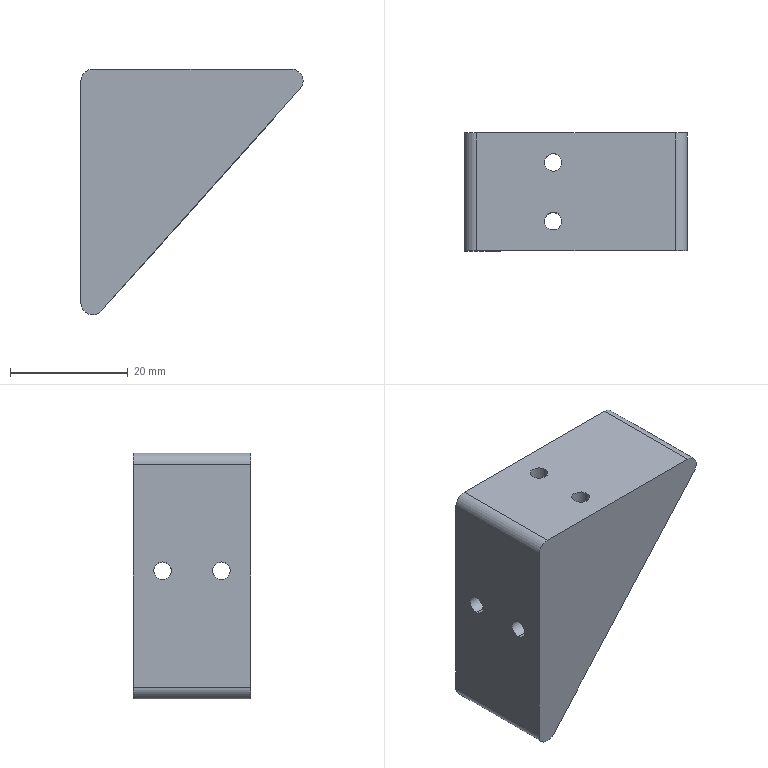Part | SolidWorks | features ICE 2, Extrusion 1, Fillet 1 | 1 solid | 25 faces | box 37.777 x 20 x 41.764 mm | volume 17216 mm3 | cylinder 20 | plane 5 | commonest cylinder face diameters 3 x16 4 x4
STEP:
#1=CARTESIAN_POINT('',(13.5,5.,-29.907));
#2=VERTEX_POINT('',#1);
#3=CARTESIAN_POINT('',(16.5,5.,-26.552));
#4=VERTEX_POINT('',#3);
#5=CARTESIAN_POINT('',(13.5,5.,-29.907));
#6=CARTESIAN_POINT('',(13.5,2.,-29.907));
#7=CARTESIAN_POINT('',(16.5,2.,-26.552));
#8=CARTESIAN_POINT('',(16.5,5.,-26.552));
#9=(BOUNDED_CURVE()B_SPLINE_CURVE(3,(#5,#6,#7,#8),.UNSPECIFIED.,.F.,.F.)B_SPLINE_CURVE_WITH_KNOTS((4,4),(3.142,6.283),.UNSPECIFIED.)CURVE()GEOMETRIC_REPRESENTATION_ITEM()RATIONAL_B_SPLINE_CURVE((1.,0.3333,0.3333,1.))REPRESENTATION_ITEM(''));
#10=EDGE_CURVE('',#2,#4,#9,.T.);
#11=ORIENTED_EDGE('',*,*,#10,.F.);
#12=CARTESIAN_POINT('',(13.5,5.,-21.5));
#13=VERTEX_POINT('',#12);
#14=CARTESIAN_POINT('',(13.5,5.,-41.764));
#15=DIRECTION('',(0.,0.,1.));
#16=VECTOR('',#15,1000.);
#17=LINE('',#14,#16);
#18=EDGE_CURVE('',#2,#13,#17,.T.);
#19=ORIENTED_EDGE('',*,*,#18,.T.);
#20=CARTESIAN_POINT('',(15.,3.5,-20.));
#21=VERTEX_POINT('',#20);
#22=CARTESIAN_POINT('',(15.,3.5,-20.));
#23=CARTESIAN_POINT('',(14.121,3.5,-20.879));
#24=CARTESIAN_POINT('',(13.5,4.121,-21.5));
#25=CARTESIAN_POINT('',(13.5,5.,-21.5));
#26=(BOUNDED_CURVE()B_SPLINE_CURVE(3,(#22,#23,#24,#25),.UNSPECIFIED.,.F.,.F.)B_SPLINE_CURVE_WITH_KNOTS((4,4),(4.712,6.283),.UNSPECIFIED.)CURVE()GEOMETRIC_REPRESENTATION_ITEM()RATIONAL_B_SPLINE_CURVE((1.,0.8047,0.8047,1.))REPRESENTATION_ITEM(''));
#27=EDGE_CURVE('',#21,#13,#26,.T.);
#28=ORIENTED_EDGE('',*,*,#27,.F.);
#29=CARTESIAN_POINT('',(16.5,5.,-21.5));
#30=VERTEX_POINT('',#29);
#31=CARTESIAN_POINT('',(16.5,5.,-21.5));
#32=CARTESIAN_POINT('',(16.5,4.121,-21.5));
#33=CARTESIAN_POINT('',(15.879,3.5,-20.879));
#34=CARTESIAN_POINT('',(15.,3.5,-20.));
#35=(BOUNDED_CURVE()B_SPLINE_CURVE(3,(#31,#32,#33,#34),.UNSPECIFIED.,.F.,.F.)B_SPLINE_CURVE_WITH_KNOTS((4,4),(3.142,4.712),.UNSPECIFIED.)CURVE()GEOMETRIC_REPRESENTATION_ITEM()RATIONAL_B_SPLINE_CURVE((1.,0.8047,0.8047,1.))REPRESENTATION_ITEM(''));
#36=EDGE_CURVE('',#30,#21,#35,.T.);
#37=ORIENTED_EDGE('',*,*,#36,.F.);
#38=CARTESIAN_POINT('',(16.5,5.,-41.764));
#39=DIRECTION('',(0.,0.,1.));
#40=VECTOR('',#39,1000.);
#41=LINE('',#38,#40);
#42=EDGE_CURVE('',#4,#30,#41,.T.);
#43=ORIENTED_EDGE('',*,*,#42,.F.);
#44=EDGE_LOOP('',(#11,#19,#28,#37,#43));
#45=FACE_OUTER_BOUND('',#44,.T.);
#46=CARTESIAN_POINT('',(15.,5.,-41.764));
#47=DIRECTION('',(0.,0.,1.));
#48=DIRECTION('',(1.,0.,0.));
#49=AXIS2_PLACEMENT_3D('',#46,#47,#48);
#50=CYLINDRICAL_SURFACE('',#49,1.5);
#51=ADVANCED_FACE('',(#45),#50,.F.);
#52=CARTESIAN_POINT('',(13.5,5.,-18.5));
#53=VERTEX_POINT('',#52);
#54=CARTESIAN_POINT('',(13.5,5.,-18.5));
#55=CARTESIAN_POINT('',(13.5,4.121,-18.5));
#56=CARTESIAN_POINT('',(14.121,3.5,-19.121));
#57=CARTESIAN_POINT('',(15.,3.5,-20.));
#58=(BOUNDED_CURVE()B_SPLINE_CURVE(3,(#54,#55,#56,#57),.UNSPECIFIED.,.F.,.F.)B_SPLINE_CURVE_WITH_KNOTS((4,4),(0.,1.571),.UNSPECIFIED.)CURVE()GEOMETRIC_REPRESENTATION_ITEM()RATIONAL_B_SPLINE_CURVE((1.,0.8047,0.8047,1.))REPRESENTATION_ITEM(''));
#59=EDGE_CURVE('',#53,#21,#58,.T.);
#60=ORIENTED_EDGE('',*,*,#59,.F.);
#61=CARTESIAN_POINT('',(13.5,5.,0.));
#62=VERTEX_POINT('',#61);
#63=CARTESIAN_POINT('',(13.5,5.,-41.764));
#64=DIRECTION('',(0.,0.,1.));
#65=VECTOR('',#64,1000.);
#66=LINE('',#63,#65);
#67=EDGE_CURVE('',#53,#62,#66,.T.);
#68=ORIENTED_EDGE('',*,*,#67,.T.);
#69=CARTESIAN_POINT('',(16.5,5.,0.));
#70=VERTEX_POINT('',#69);
#71=CARTESIAN_POINT('',(15.,5.,0.));
#72=DIRECTION('',(0.,0.,1.));
#73=DIRECTION('',(1.,0.,0.));
#74=AXIS2_PLACEMENT_3D('',#71,#72,#73);
#75=CIRCLE('',#74,1.5);
#76=EDGE_CURVE('',#62,#70,#75,.T.);
#77=ORIENTED_EDGE('',*,*,#76,.T.);
#78=CARTESIAN_POINT('',(16.5,5.,-18.5));
#79=VERTEX_POINT('',#78);
#80=CARTESIAN_POINT('',(16.5,5.,-41.764));
#81=DIRECTION('',(0.,0.,1.));
#82=VECTOR('',#81,1000.);
#83=LINE('',#80,#82);
#84=EDGE_CURVE('',#79,#70,#83,.T.);
#85=ORIENTED_EDGE('',*,*,#84,.F.);
#86=CARTESIAN_POINT('',(15.,3.5,-20.));
#87=CARTESIAN_POINT('',(15.879,3.5,-19.121));
#88=CARTESIAN_POINT('',(16.5,4.121,-18.5));
#89=CARTESIAN_POINT('',(16.5,5.,-18.5));
#90=(BOUNDED_CURVE()B_SPLINE_CURVE(3,(#86,#87,#88,#89),.UNSPECIFIED.,.F.,.F.)B_SPLINE_CURVE_WITH_KNOTS((4,4),(1.571,3.142),.UNSPECIFIED.)CURVE()GEOMETRIC_REPRESENTATION_ITEM()RATIONAL_B_SPLINE_CURVE((1.,0.8047,0.8047,1.))REPRESENTATION_ITEM(''));
#91=EDGE_CURVE('',#21,#79,#90,.T.);
#92=ORIENTED_EDGE('',*,*,#91,.F.);
#93=EDGE_LOOP('',(#60,#68,#77,#85,#92));
#94=FACE_OUTER_BOUND('',#93,.T.);
#95=CARTESIAN_POINT('',(15.,5.,-41.764));
#96=DIRECTION('',(0.,0.,1.));
#97=DIRECTION('',(1.,0.,0.));
#98=AXIS2_PLACEMENT_3D('',#95,#96,#97);
#99=CYLINDRICAL_SURFACE('',#98,1.5);
#100=ADVANCED_FACE('',(#94),#99,.F.);
#101=CARTESIAN_POINT('',(13.5,15.,-29.907));
#102=VERTEX_POINT('',#101);
#103=CARTESIAN_POINT('',(16.5,15.,-26.552));
#104=VERTEX_POINT('',#103);
#105=CARTESIAN_POINT('',(13.5,15.,-29.907));
#106=CARTESIAN_POINT('',(13.5,12.,-29.907));
#107=CARTESIAN_POINT('',(16.5,12.,-26.552));
#108=CARTESIAN_POINT('',(16.5,15.,-26.552));
#109=(BOUNDED_CURVE()B_SPLINE_CURVE(3,(#105,#106,#107,#108),.UNSPECIFIED.,.F.,.F.)B_SPLINE_CURVE_WITH_KNOTS((4,4),(3.142,6.283),.UNSPECIFIED.)CURVE()GEOMETRIC_REPRESENTATION_ITEM()RATIONAL_B_SPLINE_CURVE((1.,0.3333,0.3333,1.))REPRESENTATION_ITEM(''));
#110=EDGE_CURVE('',#102,#104,#109,.T.);
#111=ORIENTED_EDGE('',*,*,#110,.F.);
#112=CARTESIAN_POINT('',(13.5,15.,-21.5));
#113=VERTEX_POINT('',#112);
#114=CARTESIAN_POINT('',(13.5,15.,-41.764));
#115=DIRECTION('',(0.,0.,1.));
#116=VECTOR('',#115,1000.);
#117=LINE('',#114,#116);
#118=EDGE_CURVE('',#102,#113,#117,.T.);
#119=ORIENTED_EDGE('',*,*,#118,.T.);
#120=CARTESIAN_POINT('',(15.,13.5,-20.));
#121=VERTEX_POINT('',#120);
#122=CARTESIAN_POINT('',(15.,13.5,-20.));
#123=CARTESIAN_POINT('',(14.121,13.5,-20.879));
#124=CARTESIAN_POINT('',(13.5,14.121,-21.5));
#125=CARTESIAN_POINT('',(13.5,15.,-21.5));
#126=(BOUNDED_CURVE()B_SPLINE_CURVE(3,(#122,#123,#124,#125),.UNSPECIFIED.,.F.,.F.)B_SPLINE_CURVE_WITH_KNOTS((4,4),(4.712,6.283),.UNSPECIFIED.)CURVE()GEOMETRIC_REPRESENTATION_ITEM()RATIONAL_B_SPLINE_CURVE((1.,0.8047,0.8047,1.))REPRESENTATION_ITEM(''));
#127=EDGE_CURVE('',#121,#113,#126,.T.);
#128=ORIENTED_EDGE('',*,*,#127,.F.);
#129=CARTESIAN_POINT('',(16.5,15.,-21.5));
#130=VERTEX_POINT('',#129);
#131=CARTESIAN_POINT('',(16.5,15.,-21.5));
#132=CARTESIAN_POINT('',(16.5,14.121,-21.5));
#133=CARTESIAN_POINT('',(15.879,13.5,-20.879));
#134=CARTESIAN_POINT('',(15.,13.5,-20.));
#135=(BOUNDED_CURVE()B_SPLINE_CURVE(3,(#131,#132,#133,#134),.UNSPECIFIED.,.F.,.F.)B_SPLINE_CURVE_WITH_KNOTS((4,4),(3.142,4.712),.UNSPECIFIED.)CURVE()GEOMETRIC_REPRESENTATION_ITEM()RATIONAL_B_SPLINE_CURVE((1.,0.8047,0.8047,1.))REPRESENTATION_ITEM(''));
#136=EDGE_CURVE('',#130,#121,#135,.T.);
#137=ORIENTED_EDGE('',*,*,#136,.F.);
#138=CARTESIAN_POINT('',(16.5,15.,-41.764));
#139=DIRECTION('',(0.,0.,1.));
#140=VECTOR('',#139,1000.);
#141=LINE('',#138,#140);
#142=EDGE_CURVE('',#104,#130,#141,.T.);
#143=ORIENTED_EDGE('',*,*,#142,.F.);
#144=EDGE_LOOP('',(#111,#119,#128,#137,#143));
#145=FACE_OUTER_BOUND('',#144,.T.);
#146=CARTESIAN_POINT('',(15.,15.,-41.764));
#147=DIRECTION('',(0.,0.,1.));
#148=DIRECTION('',(1.,0.,0.));
#149=AXIS2_PLACEMENT_3D('',#146,#147,#148);
#150=CYLINDRICAL_SURFACE('',#149,1.5);
#151=ADVANCED_FACE('',(#145),#150,.F.);
#152=CARTESIAN_POINT('',(13.5,15.,-18.5));
#153=VERTEX_POINT('',#152);
#154=CARTESIAN_POINT('',(13.5,15.,-18.5));
#155=CARTESIAN_POINT('',(13.5,14.121,-18.5));
#156=CARTESIAN_POINT('',(14.121,13.5,-19.121));
#157=CARTESIAN_POINT('',(15.,13.5,-20.));
#158=(BOUNDED_CURVE()B_SPLINE_CURVE(3,(#154,#155,#156,#157),.UNSPECIFIED.,.F.,.F.)B_SPLINE_CURVE_WITH_KNOTS((4,4),(0.,1.571),.UNSPECIFIED.)CURVE()GEOMETRIC_REPRESENTATION_ITEM()RATIONAL_B_SPLINE_CURVE((1.,0.8047,0.8047,1.))REPRESENTATION_ITEM(''));
#159=EDGE_CURVE('',#153,#121,#158,.T.);
#160=ORIENTED_EDGE('',*,*,#159,.F.);
#161=CARTESIAN_POINT('',(13.5,15.,0.));
#162=VERTEX_POINT('',#161);
#163=CARTESIAN_POINT('',(13.5,15.,-41.764));
#164=DIRECTION('',(0.,0.,1.));
#165=VECTOR('',#164,1000.);
#166=LINE('',#163,#165);
#167=EDGE_CURVE('',#153,#162,#166,.T.);
#168=ORIENTED_EDGE('',*,*,#167,.T.);
#169=CARTESIAN_POINT('',(16.5,15.,0.));
#170=VERTEX_POINT('',#169);
#171=CARTESIAN_POINT('',(15.,15.,0.));
#172=DIRECTION('',(0.,0.,1.));
#173=DIRECTION('',(1.,0.,0.));
#174=AXIS2_PLACEMENT_3D('',#171,#172,#173);
#175=CIRCLE('',#174,1.5);
#176=EDGE_CURVE('',#162,#170,#175,.T.);
#177=ORIENTED_EDGE('',*,*,#176,.T.);
#178=CARTESIAN_POINT('',(16.5,15.,-18.5));
#179=VERTEX_POINT('',#178);
#180=CARTESIAN_POINT('',(16.5,15.,-41.764));
#181=DIRECTION('',(0.,0.,1.));
#182=VECTOR('',#181,1000.);
#183=LINE('',#180,#182);
#184=EDGE_CURVE('',#179,#170,#183,.T.);
#185=ORIENTED_EDGE('',*,*,#184,.F.);
#186=CARTESIAN_POINT('',(15.,13.5,-20.));
#187=CARTESIAN_POINT('',(15.879,13.5,-19.121));
#188=CARTESIAN_POINT('',(16.5,14.121,-18.5));
#189=CARTESIAN_POINT('',(16.5,15.,-18.5));
#190=(BOUNDED_CURVE()B_SPLINE_CURVE(3,(#186,#187,#188,#189),.UNSPECIFIED.,.F.,.F.)B_SPLINE_CURVE_WITH_KNOTS((4,4),(1.571,3.142),.UNSPECIFIED.)CURVE()GEOMETRIC_REPRESENTATION_ITEM()RATIONAL_B_SPLINE_CURVE((1.,0.8047,0.8047,1.))REPRESENTATION_ITEM(''));
#191=EDGE_CURVE('',#121,#179,#190,.T.);
#192=ORIENTED_EDGE('',*,*,#191,.F.);
#193=EDGE_LOOP('',(#160,#168,#177,#185,#192));
#194=FACE_OUTER_BOUND('',#193,.T.);
#195=CARTESIAN_POINT('',(15.,15.,-41.764));
#196=DIRECTION('',(0.,0.,1.));
#197=DIRECTION('',(1.,0.,0.));
#198=AXIS2_PLACEMENT_3D('',#195,#196,#197);
#199=CYLINDRICAL_SURFACE('',#198,1.5);
#200=ADVANCED_FACE('',(#194),#199,.F.);
#201=CARTESIAN_POINT('',(21.019,15.,-21.5));
#202=VERTEX_POINT('',#201);
#203=CARTESIAN_POINT('',(23.702,15.,-18.5));
#204=VERTEX_POINT('',#203);
#205=CARTESIAN_POINT('',(21.019,15.,-21.5));
#206=CARTESIAN_POINT('',(21.019,12.,-21.5));
#207=CARTESIAN_POINT('',(23.702,12.,-18.5));
#208=CARTESIAN_POINT('',(23.702,15.,-18.5));
#209=(BOUNDED_CURVE()B_SPLINE_CURVE(3,(#205,#206,#207,#208),.UNSPECIFIED.,.F.,.T.)B_SPLINE_CURVE_WITH_KNOTS((4,4),(0.,3.142),.UNSPECIFIED.)CURVE()GEOMETRIC_REPRESENTATION_ITEM()RATIONAL_B_SPLINE_CURVE((1.,0.3333,0.3333,1.))REPRESENTATION_ITEM(''));
#210=EDGE_CURVE('',#202,#204,#209,.T.);
#211=ORIENTED_EDGE('',*,*,#210,.F.);
#212=CARTESIAN_POINT('',(37.777,15.,-21.5));
#213=DIRECTION('',(-1.,0.,0.));
#214=VECTOR('',#213,1000.);
#215=LINE('',#212,#214);
#216=EDGE_CURVE('',#202,#130,#215,.T.);
#217=ORIENTED_EDGE('',*,*,#216,.T.);
#218=ORIENTED_EDGE('',*,*,#136,.T.);
#219=ORIENTED_EDGE('',*,*,#191,.T.);
#220=CARTESIAN_POINT('',(37.777,15.,-18.5));
#221=DIRECTION('',(-1.,0.,0.));
#222=VECTOR('',#221,1000.);
#223=LINE('',#220,#222);
#224=EDGE_CURVE('',#204,#179,#223,.T.);
#225=ORIENTED_EDGE('',*,*,#224,.F.);
#226=EDGE_LOOP('',(#211,#217,#218,#219,#225));
#227=FACE_OUTER_BOUND('',#226,.T.);
#228=CARTESIAN_POINT('',(37.777,15.,-20.));
#229=DIRECTION('',(-1.,0.,0.));
#230=DIRECTION('',(0.,0.,1.));
#231=AXIS2_PLACEMENT_3D('',#228,#229,#230);
#232=CYLINDRICAL_SURFACE('',#231,1.5);
#233=ADVANCED_FACE('',(#227),#232,.F.);
#234=CARTESIAN_POINT('',(21.019,5.,-21.5));
#235=VERTEX_POINT('',#234);
#236=CARTESIAN_POINT('',(23.702,5.,-18.5));
#237=VERTEX_POINT('',#236);
#238=CARTESIAN_POINT('',(21.019,5.,-21.5));
#239=CARTESIAN_POINT('',(21.019,2.,-21.5));
#240=CARTESIAN_POINT('',(23.702,2.,-18.5));
#241=CARTESIAN_POINT('',(23.702,5.,-18.5));
#242=(BOUNDED_CURVE()B_SPLINE_CURVE(3,(#238,#239,#240,#241),.UNSPECIFIED.,.F.,.F.)B_SPLINE_CURVE_WITH_KNOTS((4,4),(0.,3.142),.UNSPECIFIED.)CURVE()GEOMETRIC_REPRESENTATION_ITEM()RATIONAL_B_SPLINE_CURVE((1.,0.3333,0.3333,1.))REPRESENTATION_ITEM(''));
#243=EDGE_CURVE('',#235,#237,#242,.T.);
#244=ORIENTED_EDGE('',*,*,#243,.F.);
#245=CARTESIAN_POINT('',(37.777,5.,-21.5));
#246=DIRECTION('',(-1.,0.,0.));
#247=VECTOR('',#246,1000.);
#248=LINE('',#245,#247);
#249=EDGE_CURVE('',#235,#30,#248,.T.);
#250=ORIENTED_EDGE('',*,*,#249,.T.);
#251=ORIENTED_EDGE('',*,*,#36,.T.);
#252=ORIENTED_EDGE('',*,*,#91,.T.);
#253=CARTESIAN_POINT('',(37.777,5.,-18.5));
#254=DIRECTION('',(-1.,0.,0.));
#255=VECTOR('',#254,1000.);
#256=LINE('',#253,#255);
#257=EDGE_CURVE('',#237,#79,#256,.T.);
#258=ORIENTED_EDGE('',*,*,#257,.F.);
#259=EDGE_LOOP('',(#244,#250,#251,#252,#258));
#260=FACE_OUTER_BOUND('',#259,.T.);
#261=CARTESIAN_POINT('',(37.777,5.,-20.));
#262=DIRECTION('',(-1.,0.,0.));
#263=DIRECTION('',(0.,0.,1.));
#264=AXIS2_PLACEMENT_3D('',#261,#262,#263);
#265=CYLINDRICAL_SURFACE('',#264,1.5);
#266=ADVANCED_FACE('',(#260),#265,.F.);
#267=CARTESIAN_POINT('',(2.,20.,-41.764));
#268=VERTEX_POINT('',#267);
#269=CARTESIAN_POINT('',(0.,20.,-39.764));
#270=VERTEX_POINT('',#269);
#271=CARTESIAN_POINT('',(2.,20.,-39.764));
#272=DIRECTION('',(0.,1.,0.));
#273=DIRECTION('',(0.,0.,-1.));
#274=AXIS2_PLACEMENT_3D('',#271,#272,#273);
#275=CIRCLE('',#274,2.);
#276=EDGE_CURVE('',#268,#270,#275,.T.);
#277=ORIENTED_EDGE('',*,*,#276,.F.);
#278=CARTESIAN_POINT('',(2.,0.,-41.764));
#279=VERTEX_POINT('',#278);
#280=CARTESIAN_POINT('',(2.,20.,-41.764));
#281=DIRECTION('',(0.,-1.,0.));
#282=VECTOR('',#281,1000.);
#283=LINE('',#280,#282);
#284=EDGE_CURVE('',#268,#279,#283,.T.);
#285=ORIENTED_EDGE('',*,*,#284,.T.);
#286=CARTESIAN_POINT('',(0.,0.,-39.764));
#287=VERTEX_POINT('',#286);
#288=CARTESIAN_POINT('',(2.,0.,-39.764));
#289=DIRECTION('',(0.,-1.,0.));
#290=DIRECTION('',(0.,0.,-1.));
#291=AXIS2_PLACEMENT_3D('',#288,#289,#290);
#292=CIRCLE('',#291,2.);
#293=EDGE_CURVE('',#287,#279,#292,.T.);
#294=ORIENTED_EDGE('',*,*,#293,.F.);
#295=CARTESIAN_POINT('',(0.,20.,-39.764));
#296=DIRECTION('',(0.,-1.,0.));
#297=VECTOR('',#296,1000.);
#298=LINE('',#295,#297);
#299=EDGE_CURVE('',#270,#287,#298,.T.);
#300=ORIENTED_EDGE('',*,*,#299,.F.);
#301=EDGE_LOOP('',(#277,#285,#294,#300));
#302=FACE_OUTER_BOUND('',#301,.T.);
#303=CARTESIAN_POINT('',(2.,20.,-39.764));
#304=DIRECTION('',(0.,-1.,0.));
#305=DIRECTION('',(0.,0.,-1.));
#306=AXIS2_PLACEMENT_3D('',#303,#304,#305);
#307=CYLINDRICAL_SURFACE('',#306,2.);
#308=ADVANCED_FACE('',(#302),#307,.T.);
#309=ORIENTED_EDGE('',*,*,#127,.T.);
#310=CARTESIAN_POINT('',(0.,15.,-21.5));
#311=VERTEX_POINT('',#310);
#312=CARTESIAN_POINT('',(37.777,15.,-21.5));
#313=DIRECTION('',(-1.,0.,0.));
#314=VECTOR('',#313,1000.);
#315=LINE('',#312,#314);
#316=EDGE_CURVE('',#113,#311,#315,.T.);
#317=ORIENTED_EDGE('',*,*,#316,.T.);
#318=CARTESIAN_POINT('',(0.,15.,-18.5));
#319=VERTEX_POINT('',#318);
#320=CARTESIAN_POINT('',(0.,15.,-20.));
#321=DIRECTION('',(-1.,0.,0.));
#322=DIRECTION('',(0.,0.,1.));
#323=AXIS2_PLACEMENT_3D('',#320,#321,#322);
#324=CIRCLE('',#323,1.5);
#325=EDGE_CURVE('',#311,#319,#324,.T.);
#326=ORIENTED_EDGE('',*,*,#325,.T.);
#327=CARTESIAN_POINT('',(37.777,15.,-18.5));
#328=DIRECTION('',(-1.,0.,0.));
#329=VECTOR('',#328,1000.);
#330=LINE('',#327,#329);
#331=EDGE_CURVE('',#153,#319,#330,.T.);
#332=ORIENTED_EDGE('',*,*,#331,.F.);
#333=ORIENTED_EDGE('',*,*,#159,.T.);
#334=EDGE_LOOP('',(#309,#317,#326,#332,#333));
#335=FACE_OUTER_BOUND('',#334,.T.);
#336=CARTESIAN_POINT('',(37.777,15.,-20.));
#337=DIRECTION('',(-1.,0.,0.));
#338=DIRECTION('',(0.,0.,1.));
#339=AXIS2_PLACEMENT_3D('',#336,#337,#338);
#340=CYLINDRICAL_SURFACE('',#339,1.5);
#341=ADVANCED_FACE('',(#335),#340,.F.);
#342=ORIENTED_EDGE('',*,*,#27,.T.);
#343=CARTESIAN_POINT('',(0.,5.,-21.5));
#344=VERTEX_POINT('',#343);
#345=CARTESIAN_POINT('',(37.777,5.,-21.5));
#346=DIRECTION('',(-1.,0.,0.));
#347=VECTOR('',#346,1000.);
#348=LINE('',#345,#347);
#349=EDGE_CURVE('',#13,#344,#348,.T.);
#350=ORIENTED_EDGE('',*,*,#349,.T.);
#351=CARTESIAN_POINT('',(0.,5.,-18.5));
#352=VERTEX_POINT('',#351);
#353=CARTESIAN_POINT('',(0.,5.,-20.));
#354=DIRECTION('',(-1.,0.,0.));
#355=DIRECTION('',(0.,0.,1.));
#356=AXIS2_PLACEMENT_3D('',#353,#354,#355);
#357=CIRCLE('',#356,1.5);
#358=EDGE_CURVE('',#344,#352,#357,.T.);
#359=ORIENTED_EDGE('',*,*,#358,.T.);
#360=CARTESIAN_POINT('',(37.777,5.,-18.5));
#361=DIRECTION('',(-1.,0.,0.));
#362=VECTOR('',#361,1000.);
#363=LINE('',#360,#362);
#364=EDGE_CURVE('',#53,#352,#363,.T.);
#365=ORIENTED_EDGE('',*,*,#364,.F.);
#366=ORIENTED_EDGE('',*,*,#59,.T.);
#367=EDGE_LOOP('',(#342,#350,#359,#365,#366));
#368=FACE_OUTER_BOUND('',#367,.T.);
#369=CARTESIAN_POINT('',(37.777,5.,-20.));
#370=DIRECTION('',(-1.,0.,0.));
#371=DIRECTION('',(0.,0.,1.));
#372=AXIS2_PLACEMENT_3D('',#369,#370,#371);
#373=CYLINDRICAL_SURFACE('',#372,1.5);
#374=ADVANCED_FACE('',(#368),#373,.F.);
#375=ORIENTED_EDGE('',*,*,#349,.F.);
#376=CARTESIAN_POINT('',(15.,6.5,-20.));
#377=VERTEX_POINT('',#376);
#378=CARTESIAN_POINT('',(13.5,5.,-21.5));
#379=CARTESIAN_POINT('',(13.5,5.879,-21.5));
#380=CARTESIAN_POINT('',(14.121,6.5,-20.879));
#381=CARTESIAN_POINT('',(15.,6.5,-20.));
#382=(BOUNDED_CURVE()B_SPLINE_CURVE(3,(#378,#379,#380,#381),.UNSPECIFIED.,.F.,.F.)B_SPLINE_CURVE_WITH_KNOTS((4,4),(0.,1.571),.UNSPECIFIED.)CURVE()GEOMETRIC_REPRESENTATION_ITEM()RATIONAL_B_SPLINE_CURVE((1.,0.8047,0.8047,1.))REPRESENTATION_ITEM(''));
#383=EDGE_CURVE('',#13,#377,#382,.T.);
#384=ORIENTED_EDGE('',*,*,#383,.T.);
#385=CARTESIAN_POINT('',(15.,6.5,-20.));
#386=CARTESIAN_POINT('',(14.121,6.5,-19.121));
#387=CARTESIAN_POINT('',(13.5,5.879,-18.5));
#388=CARTESIAN_POINT('',(13.5,5.,-18.5));
#389=(BOUNDED_CURVE()B_SPLINE_CURVE(3,(#385,#386,#387,#388),.UNSPECIFIED.,.F.,.F.)B_SPLINE_CURVE_WITH_KNOTS((4,4),(4.712,6.283),.UNSPECIFIED.)CURVE()GEOMETRIC_REPRESENTATION_ITEM()RATIONAL_B_SPLINE_CURVE((1.,0.8047,0.8047,1.))REPRESENTATION_ITEM(''));
#390=EDGE_CURVE('',#377,#53,#389,.T.);
#391=ORIENTED_EDGE('',*,*,#390,.T.);
#392=ORIENTED_EDGE('',*,*,#364,.T.);
#393=CARTESIAN_POINT('',(0.,5.,-20.));
#394=DIRECTION('',(-1.,0.,0.));
#395=DIRECTION('',(0.,0.,1.));
#396=AXIS2_PLACEMENT_3D('',#393,#394,#395);
#397=CIRCLE('',#396,1.5);
#398=EDGE_CURVE('',#352,#344,#397,.T.);
#399=ORIENTED_EDGE('',*,*,#398,.T.);
#400=EDGE_LOOP('',(#375,#384,#391,#392,#399));
#401=FACE_OUTER_BOUND('',#400,.T.);
#402=CARTESIAN_POINT('',(37.777,5.,-20.));
#403=DIRECTION('',(-1.,0.,0.));
#404=DIRECTION('',(0.,0.,1.));
#405=AXIS2_PLACEMENT_3D('',#402,#403,#404);
#406=CYLINDRICAL_SURFACE('',#405,1.5);
#407=ADVANCED_FACE('',(#401),#406,.F.);
#408=ORIENTED_EDGE('',*,*,#316,.F.);
#409=CARTESIAN_POINT('',(15.,16.5,-20.));
#410=VERTEX_POINT('',#409);
#411=CARTESIAN_POINT('',(13.5,15.,-21.5));
#412=CARTESIAN_POINT('',(13.5,15.879,-21.5));
#413=CARTESIAN_POINT('',(14.121,16.5,-20.879));
#414=CARTESIAN_POINT('',(15.,16.5,-20.));
#415=(BOUNDED_CURVE()B_SPLINE_CURVE(3,(#411,#412,#413,#414),.UNSPECIFIED.,.F.,.F.)B_SPLINE_CURVE_WITH_KNOTS((4,4),(0.,1.571),.UNSPECIFIED.)CURVE()GEOMETRIC_REPRESENTATION_ITEM()RATIONAL_B_SPLINE_CURVE((1.,0.8047,0.8047,1.))REPRESENTATION_ITEM(''));
#416=EDGE_CURVE('',#113,#410,#415,.T.);
#417=ORIENTED_EDGE('',*,*,#416,.T.);
#418=CARTESIAN_POINT('',(15.,16.5,-20.));
#419=CARTESIAN_POINT('',(14.121,16.5,-19.121));
#420=CARTESIAN_POINT('',(13.5,15.879,-18.5));
#421=CARTESIAN_POINT('',(13.5,15.,-18.5));
#422=(BOUNDED_CURVE()B_SPLINE_CURVE(3,(#418,#419,#420,#421),.UNSPECIFIED.,.F.,.F.)B_SPLINE_CURVE_WITH_KNOTS((4,4),(4.712,6.283),.UNSPECIFIED.)CURVE()GEOMETRIC_REPRESENTATION_ITEM()RATIONAL_B_SPLINE_CURVE((1.,0.8047,0.8047,1.))REPRESENTATION_ITEM(''));
#423=EDGE_CURVE('',#410,#153,#422,.T.);
#424=ORIENTED_EDGE('',*,*,#423,.T.);
#425=ORIENTED_EDGE('',*,*,#331,.T.);
#426=CARTESIAN_POINT('',(0.,15.,-20.));
#427=DIRECTION('',(-1.,0.,0.));
#428=DIRECTION('',(0.,0.,1.));
#429=AXIS2_PLACEMENT_3D('',#426,#427,#428);
#430=CIRCLE('',#429,1.5);
#431=EDGE_CURVE('',#319,#311,#430,.T.);
#432=ORIENTED_EDGE('',*,*,#431,.T.);
#433=EDGE_LOOP('',(#408,#417,#424,#425,#432));
#434=FACE_OUTER_BOUND('',#433,.T.);
#435=CARTESIAN_POINT('',(37.777,15.,-20.));
#436=DIRECTION('',(-1.,0.,0.));
#437=DIRECTION('',(0.,0.,1.));
#438=AXIS2_PLACEMENT_3D('',#435,#436,#437);
#439=CYLINDRICAL_SURFACE('',#438,1.5);
#440=ADVANCED_FACE('',(#434),#439,.F.);
#441=CARTESIAN_POINT('',(16.5,15.,-26.552));
#442=CARTESIAN_POINT('',(16.5,18.,-26.552));
#443=CARTESIAN_POINT('',(13.5,18.,-29.907));
#444=CARTESIAN_POINT('',(13.5,15.,-29.907));
#445=(BOUNDED_CURVE()B_SPLINE_CURVE(3,(#441,#442,#443,#444),.UNSPECIFIED.,.F.,.F.)B_SPLINE_CURVE_WITH_KNOTS((4,4),(0.,3.142),.UNSPECIFIED.)CURVE()GEOMETRIC_REPRESENTATION_ITEM()RATIONAL_B_SPLINE_CURVE((1.,0.3333,0.3333,1.))REPRESENTATION_ITEM(''));
#446=EDGE_CURVE('',#104,#102,#445,.T.);
#447=ORIENTED_EDGE('',*,*,#446,.T.);
#448=ORIENTED_EDGE('',*,*,#110,.T.);
#449=EDGE_LOOP('',(#447,#448));
#450=FACE_BOUND('',#449,.T.);
#451=CARTESIAN_POINT('',(16.5,5.,-26.552));
#452=CARTESIAN_POINT('',(16.5,8.,-26.552));
#453=CARTESIAN_POINT('',(13.5,8.,-29.907));
#454=CARTESIAN_POINT('',(13.5,5.,-29.907));
#455=(BOUNDED_CURVE()B_SPLINE_CURVE(3,(#451,#452,#453,#454),.UNSPECIFIED.,.F.,.F.)B_SPLINE_CURVE_WITH_KNOTS((4,4),(0.,3.142),.UNSPECIFIED.)CURVE()GEOMETRIC_REPRESENTATION_ITEM()RATIONAL_B_SPLINE_CURVE((1.,0.3333,0.3333,1.))REPRESENTATION_ITEM(''));
#456=EDGE_CURVE('',#4,#2,#455,.T.);
#457=ORIENTED_EDGE('',*,*,#456,.T.);
#458=ORIENTED_EDGE('',*,*,#10,.T.);
#459=EDGE_LOOP('',(#457,#458));
#460=FACE_BOUND('',#459,.T.);
#461=CARTESIAN_POINT('',(23.702,15.,-18.5));
#462=CARTESIAN_POINT('',(23.702,18.,-18.5));
#463=CARTESIAN_POINT('',(21.019,18.,-21.5));
#464=CARTESIAN_POINT('',(21.019,15.,-21.5));
#465=(BOUNDED_CURVE()B_SPLINE_CURVE(3,(#461,#462,#463,#464),.UNSPECIFIED.,.F.,.F.)B_SPLINE_CURVE_WITH_KNOTS((4,4),(3.142,6.283),.UNSPECIFIED.)CURVE()GEOMETRIC_REPRESENTATION_ITEM()RATIONAL_B_SPLINE_CURVE((1.,0.3333,0.3333,1.))REPRESENTATION_ITEM(''));
#466=EDGE_CURVE('',#204,#202,#465,.T.);
#467=ORIENTED_EDGE('',*,*,#466,.T.);
#468=ORIENTED_EDGE('',*,*,#210,.T.);
#469=EDGE_LOOP('',(#467,#468));
#470=FACE_BOUND('',#469,.T.);
#471=CARTESIAN_POINT('',(23.702,5.,-18.5));
#472=CARTESIAN_POINT('',(23.702,8.,-18.5));
#473=CARTESIAN_POINT('',(21.019,8.,-21.5));
#474=CARTESIAN_POINT('',(21.019,5.,-21.5));
#475=(BOUNDED_CURVE()B_SPLINE_CURVE(3,(#471,#472,#473,#474),.UNSPECIFIED.,.F.,.F.)B_SPLINE_CURVE_WITH_KNOTS((4,4),(3.142,6.283),.UNSPECIFIED.)CURVE()GEOMETRIC_REPRESENTATION_ITEM()RATIONAL_B_SPLINE_CURVE((1.,0.3333,0.3333,1.))REPRESENTATION_ITEM(''));
#476=EDGE_CURVE('',#237,#235,#475,.T.);
#477=ORIENTED_EDGE('',*,*,#476,.T.);
#478=ORIENTED_EDGE('',*,*,#243,.T.);
#479=EDGE_LOOP('',(#477,#478));
#480=FACE_BOUND('',#479,.T.);
#481=CARTESIAN_POINT('',(37.268,20.,-3.333));
#482=VERTEX_POINT('',#481);
#483=CARTESIAN_POINT('',(3.491,20.,-41.097));
#484=VERTEX_POINT('',#483);
#485=CARTESIAN_POINT('',(40.249,20.,0.));
#486=DIRECTION('',(-0.6667,0.,-0.7454));
#487=VECTOR('',#486,1000.);
#488=LINE('',#485,#487);
#489=EDGE_CURVE('',#482,#484,#488,.T.);
#490=ORIENTED_EDGE('',*,*,#489,.F.);
#491=CARTESIAN_POINT('',(37.268,0.,-3.333));
#492=VERTEX_POINT('',#491);
#493=CARTESIAN_POINT('',(37.268,20.,-3.333));
#494=DIRECTION('',(0.,-1.,0.));
#495=VECTOR('',#494,1000.);
#496=LINE('',#493,#495);
#497=EDGE_CURVE('',#482,#492,#496,.T.);
#498=ORIENTED_EDGE('',*,*,#497,.T.);
#499=CARTESIAN_POINT('',(3.491,0.,-41.097));
#500=VERTEX_POINT('',#499);
#501=CARTESIAN_POINT('',(40.249,0.,0.));
#502=DIRECTION('',(-0.6667,0.,-0.7454));
#503=VECTOR('',#502,1000.);
#504=LINE('',#501,#503);
#505=EDGE_CURVE('',#492,#500,#504,.T.);
#506=ORIENTED_EDGE('',*,*,#505,.T.);
#507=CARTESIAN_POINT('',(3.491,20.,-41.097));
#508=DIRECTION('',(0.,1.,0.));
#509=VECTOR('',#508,1000.);
#510=LINE('',#507,#509);
#511=EDGE_CURVE('',#500,#484,#510,.T.);
#512=ORIENTED_EDGE('',*,*,#511,.T.);
#513=EDGE_LOOP('',(#490,#498,#506,#512));
#514=FACE_OUTER_BOUND('',#513,.T.);
#515=CARTESIAN_POINT('',(40.249,20.,0.));
#516=DIRECTION('',(-0.7454,0.,0.6667));
#517=DIRECTION('',(0.6667,0.,0.7454));
#518=AXIS2_PLACEMENT_3D('',#515,#516,#517);
#519=PLANE('',#518);
#520=ADVANCED_FACE('',(#450,#460,#470,#480,#514),#519,.F.);
#521=ORIENTED_EDGE('',*,*,#431,.F.);
#522=ORIENTED_EDGE('',*,*,#325,.F.);
#523=EDGE_LOOP('',(#521,#522));
#524=FACE_BOUND('',#523,.T.);
#525=ORIENTED_EDGE('',*,*,#398,.F.);
#526=ORIENTED_EDGE('',*,*,#358,.F.);
#527=EDGE_LOOP('',(#525,#526));
#528=FACE_BOUND('',#527,.T.);
#529=CARTESIAN_POINT('',(0.,20.,-2.));
#530=VERTEX_POINT('',#529);
#531=CARTESIAN_POINT('',(0.,20.,-45.));
#532=DIRECTION('',(0.,0.,1.));
#533=VECTOR('',#532,1000.);
#534=LINE('',#531,#533);
#535=EDGE_CURVE('',#270,#530,#534,.T.);
#536=ORIENTED_EDGE('',*,*,#535,.F.);
#537=ORIENTED_EDGE('',*,*,#299,.T.);
#538=CARTESIAN_POINT('',(0.,0.,-2.));
#539=VERTEX_POINT('',#538);
#540=CARTESIAN_POINT('',(0.,0.,-45.));
#541=DIRECTION('',(0.,0.,1.));
#542=VECTOR('',#541,1000.);
#543=LINE('',#540,#542);
#544=EDGE_CURVE('',#287,#539,#543,.T.);
#545=ORIENTED_EDGE('',*,*,#544,.T.);
#546=CARTESIAN_POINT('',(0.,20.,-2.));
#547=DIRECTION('',(0.,1.,0.));
#548=VECTOR('',#547,1000.);
#549=LINE('',#546,#548);
#550=EDGE_CURVE('',#539,#530,#549,.T.);
#551=ORIENTED_EDGE('',*,*,#550,.T.);
#552=EDGE_LOOP('',(#536,#537,#545,#551));
#553=FACE_OUTER_BOUND('',#552,.T.);
#554=CARTESIAN_POINT('',(0.,20.,-45.));
#555=DIRECTION('',(1.,0.,0.));
#556=DIRECTION('',(0.,0.,-1.));
#557=AXIS2_PLACEMENT_3D('',#554,#555,#556);
#558=PLANE('',#557);
#559=ADVANCED_FACE('',(#524,#528,#553),#558,.F.);
#560=CARTESIAN_POINT('',(15.,15.,0.));
#561=DIRECTION('',(0.,0.,1.));
#562=DIRECTION('',(1.,0.,0.));
#563=AXIS2_PLACEMENT_3D('',#560,#561,#562);
#564=CIRCLE('',#563,1.5);
#565=EDGE_CURVE('',#170,#162,#564,.T.);
#566=ORIENTED_EDGE('',*,*,#565,.F.);
#567=ORIENTED_EDGE('',*,*,#176,.F.);
#568=EDGE_LOOP('',(#566,#567));
#569=FACE_BOUND('',#568,.T.);
#570=CARTESIAN_POINT('',(15.,5.,0.));
#571=DIRECTION('',(0.,0.,1.));
#572=DIRECTION('',(1.,0.,0.));
#573=AXIS2_PLACEMENT_3D('',#570,#571,#572);
#574=CIRCLE('',#573,1.5);
#575=EDGE_CURVE('',#70,#62,#574,.T.);
#576=ORIENTED_EDGE('',*,*,#575,.F.);
#577=ORIENTED_EDGE('',*,*,#76,.F.);
#578=EDGE_LOOP('',(#576,#577));
#579=FACE_BOUND('',#578,.T.);
#580=CARTESIAN_POINT('',(2.,0.,0.));
#581=VERTEX_POINT('',#580);
#582=CARTESIAN_POINT('',(35.777,0.,0.));
#583=VERTEX_POINT('',#582);
#584=CARTESIAN_POINT('',(0.,0.,0.));
#585=DIRECTION('',(1.,0.,0.));
#586=VECTOR('',#585,1000.);
#587=LINE('',#584,#586);
#588=EDGE_CURVE('',#581,#583,#587,.T.);
#589=ORIENTED_EDGE('',*,*,#588,.T.);
#590=CARTESIAN_POINT('',(35.777,20.,0.));
#591=VERTEX_POINT('',#590);
#592=CARTESIAN_POINT('',(35.777,20.,0.));
#593=DIRECTION('',(0.,1.,0.));
#594=VECTOR('',#593,1000.);
#595=LINE('',#592,#594);
#596=EDGE_CURVE('',#583,#591,#595,.T.);
#597=ORIENTED_EDGE('',*,*,#596,.T.);
#598=CARTESIAN_POINT('',(2.,20.,0.));
#599=VERTEX_POINT('',#598);
#600=CARTESIAN_POINT('',(0.,20.,0.));
#601=DIRECTION('',(1.,0.,0.));
#602=VECTOR('',#601,1000.);
#603=LINE('',#600,#602);
#604=EDGE_CURVE('',#599,#591,#603,.T.);
#605=ORIENTED_EDGE('',*,*,#604,.F.);
#606=CARTESIAN_POINT('',(2.,20.,0.));
#607=DIRECTION('',(0.,-1.,0.));
#608=VECTOR('',#607,1000.);
#609=LINE('',#606,#608);
#610=EDGE_CURVE('',#599,#581,#609,.T.);
#611=ORIENTED_EDGE('',*,*,#610,.T.);
#612=EDGE_LOOP('',(#589,#597,#605,#611));
#613=FACE_OUTER_BOUND('',#612,.T.);
#614=CARTESIAN_POINT('',(0.,20.,0.));
#615=DIRECTION('',(0.,0.,-1.));
#616=DIRECTION('',(-1.,0.,0.));
#617=AXIS2_PLACEMENT_3D('',#614,#615,#616);
#618=PLANE('',#617);
#619=ADVANCED_FACE('',(#569,#579,#613),#618,.F.);
#620=ORIENTED_EDGE('',*,*,#604,.T.);
#621=CARTESIAN_POINT('',(35.777,20.,-2.));
#622=DIRECTION('',(0.,1.,0.));
#623=DIRECTION('',(0.,0.,-1.));
#624=AXIS2_PLACEMENT_3D('',#621,#622,#623);
#625=CIRCLE('',#624,2.);
#626=EDGE_CURVE('',#591,#482,#625,.T.);
#627=ORIENTED_EDGE('',*,*,#626,.T.);
#628=ORIENTED_EDGE('',*,*,#489,.T.);
#629=CARTESIAN_POINT('',(2.,20.,-39.764));
#630=DIRECTION('',(0.,1.,0.));
#631=DIRECTION('',(0.,0.,-1.));
#632=AXIS2_PLACEMENT_3D('',#629,#630,#631);
#633=CIRCLE('',#632,2.);
#634=EDGE_CURVE('',#484,#268,#633,.T.);
#635=ORIENTED_EDGE('',*,*,#634,.T.);
#636=ORIENTED_EDGE('',*,*,#276,.T.);
#637=ORIENTED_EDGE('',*,*,#535,.T.);
#638=CARTESIAN_POINT('',(2.,20.,-2.));
#639=DIRECTION('',(0.,1.,0.));
#640=DIRECTION('',(0.,0.,-1.));
#641=AXIS2_PLACEMENT_3D('',#638,#639,#640);
#642=CIRCLE('',#641,2.);
#643=EDGE_CURVE('',#530,#599,#642,.T.);
#644=ORIENTED_EDGE('',*,*,#643,.T.);
#645=EDGE_LOOP('',(#620,#627,#628,#635,#636,#637,#644));
#646=FACE_OUTER_BOUND('',#645,.T.);
#647=CARTESIAN_POINT('',(0.,20.,0.));
#648=DIRECTION('',(0.,-1.,0.));
#649=DIRECTION('',(0.,0.,-1.));
#650=AXIS2_PLACEMENT_3D('',#647,#648,#649);
#651=PLANE('',#650);
#652=ADVANCED_FACE('',(#646),#651,.F.);
#653=ORIENTED_EDGE('',*,*,#505,.F.);
#654=CARTESIAN_POINT('',(35.777,0.,-2.));
#655=DIRECTION('',(0.,-1.,0.));
#656=DIRECTION('',(0.,0.,-1.));
#657=AXIS2_PLACEMENT_3D('',#654,#655,#656);
#658=CIRCLE('',#657,2.);
#659=EDGE_CURVE('',#492,#583,#658,.T.);
#660=ORIENTED_EDGE('',*,*,#659,.T.);
#661=ORIENTED_EDGE('',*,*,#588,.F.);
#662=CARTESIAN_POINT('',(2.,0.,-2.));
#663=DIRECTION('',(0.,-1.,0.));
#664=DIRECTION('',(0.,0.,-1.));
#665=AXIS2_PLACEMENT_3D('',#662,#663,#664);
#666=CIRCLE('',#665,2.);
#667=EDGE_CURVE('',#581,#539,#666,.T.);
#668=ORIENTED_EDGE('',*,*,#667,.T.);
#669=ORIENTED_EDGE('',*,*,#544,.F.);
#670=ORIENTED_EDGE('',*,*,#293,.T.);
#671=CARTESIAN_POINT('',(2.,0.,-39.764));
#672=DIRECTION('',(0.,-1.,0.));
#673=DIRECTION('',(0.,0.,-1.));
#674=AXIS2_PLACEMENT_3D('',#671,#672,#673);
#675=CIRCLE('',#674,2.);
#676=EDGE_CURVE('',#279,#500,#675,.T.);
#677=ORIENTED_EDGE('',*,*,#676,.T.);
#678=EDGE_LOOP('',(#653,#660,#661,#668,#669,#670,#677));
#679=FACE_OUTER_BOUND('',#678,.T.);
#680=CARTESIAN_POINT('',(0.,0.,0.));
#681=DIRECTION('',(0.,-1.,0.));
#682=DIRECTION('',(0.,0.,-1.));
#683=AXIS2_PLACEMENT_3D('',#680,#681,#682);
#684=PLANE('',#683);
#685=ADVANCED_FACE('',(#679),#684,.T.);
#686=ORIENTED_EDGE('',*,*,#626,.F.);
#687=ORIENTED_EDGE('',*,*,#596,.F.);
#688=ORIENTED_EDGE('',*,*,#659,.F.);
#689=ORIENTED_EDGE('',*,*,#497,.F.);
#690=EDGE_LOOP('',(#686,#687,#688,#689));
#691=FACE_OUTER_BOUND('',#690,.T.);
#692=CARTESIAN_POINT('',(35.777,20.,-2.));
#693=DIRECTION('',(0.,-1.,0.));
#694=DIRECTION('',(0.,0.,-1.));
#695=AXIS2_PLACEMENT_3D('',#692,#693,#694);
#696=CYLINDRICAL_SURFACE('',#695,2.);
#697=ADVANCED_FACE('',(#691),#696,.T.);
#698=ORIENTED_EDGE('',*,*,#284,.F.);
#699=ORIENTED_EDGE('',*,*,#634,.F.);
#700=ORIENTED_EDGE('',*,*,#511,.F.);
#701=ORIENTED_EDGE('',*,*,#676,.F.);
#702=EDGE_LOOP('',(#698,#699,#700,#701));
#703=FACE_OUTER_BOUND('',#702,.T.);
#704=CARTESIAN_POINT('',(2.,20.,-39.764));
#705=DIRECTION('',(0.,-1.,0.));
#706=DIRECTION('',(0.,0.,-1.));
#707=AXIS2_PLACEMENT_3D('',#704,#705,#706);
#708=CYLINDRICAL_SURFACE('',#707,2.);
#709=ADVANCED_FACE('',(#703),#708,.T.);
#710=ORIENTED_EDGE('',*,*,#643,.F.);
#711=ORIENTED_EDGE('',*,*,#550,.F.);
#712=ORIENTED_EDGE('',*,*,#667,.F.);
#713=ORIENTED_EDGE('',*,*,#610,.F.);
#714=EDGE_LOOP('',(#710,#711,#712,#713));
#715=FACE_OUTER_BOUND('',#714,.T.);
#716=CARTESIAN_POINT('',(2.,20.,-2.));
#717=DIRECTION('',(0.,-1.,0.));
#718=DIRECTION('',(0.,0.,-1.));
#719=AXIS2_PLACEMENT_3D('',#716,#717,#718);
#720=CYLINDRICAL_SURFACE('',#719,2.);
#721=ADVANCED_FACE('',(#715),#720,.T.);
#722=ORIENTED_EDGE('',*,*,#249,.F.);
#723=ORIENTED_EDGE('',*,*,#476,.F.);
#724=ORIENTED_EDGE('',*,*,#257,.T.);
#725=CARTESIAN_POINT('',(16.5,5.,-18.5));
#726=CARTESIAN_POINT('',(16.5,5.879,-18.5));
#727=CARTESIAN_POINT('',(15.879,6.5,-19.121));
#728=CARTESIAN_POINT('',(15.,6.5,-20.));
#729=(BOUNDED_CURVE()B_SPLINE_CURVE(3,(#725,#726,#727,#728),.UNSPECIFIED.,.F.,.F.)B_SPLINE_CURVE_WITH_KNOTS((4,4),(3.142,4.712),.UNSPECIFIED.)CURVE()GEOMETRIC_REPRESENTATION_ITEM()RATIONAL_B_SPLINE_CURVE((1.,0.8047,0.8047,1.))REPRESENTATION_ITEM(''));
#730=EDGE_CURVE('',#79,#377,#729,.T.);
#731=ORIENTED_EDGE('',*,*,#730,.T.);
#732=CARTESIAN_POINT('',(15.,6.5,-20.));
#733=CARTESIAN_POINT('',(15.879,6.5,-20.879));
#734=CARTESIAN_POINT('',(16.5,5.879,-21.5));
#735=CARTESIAN_POINT('',(16.5,5.,-21.5));
#736=(BOUNDED_CURVE()B_SPLINE_CURVE(3,(#732,#733,#734,#735),.UNSPECIFIED.,.F.,.F.)B_SPLINE_CURVE_WITH_KNOTS((4,4),(1.571,3.142),.UNSPECIFIED.)CURVE()GEOMETRIC_REPRESENTATION_ITEM()RATIONAL_B_SPLINE_CURVE((1.,0.8047,0.8047,1.))REPRESENTATION_ITEM(''));
#737=EDGE_CURVE('',#377,#30,#736,.T.);
#738=ORIENTED_EDGE('',*,*,#737,.T.);
#739=EDGE_LOOP('',(#722,#723,#724,#731,#738));
#740=FACE_OUTER_BOUND('',#739,.T.);
#741=CARTESIAN_POINT('',(37.777,5.,-20.));
#742=DIRECTION('',(-1.,0.,0.));
#743=DIRECTION('',(0.,0.,1.));
#744=AXIS2_PLACEMENT_3D('',#741,#742,#743);
#745=CYLINDRICAL_SURFACE('',#744,1.5);
#746=ADVANCED_FACE('',(#740),#745,.F.);
#747=ORIENTED_EDGE('',*,*,#216,.F.);
#748=ORIENTED_EDGE('',*,*,#466,.F.);
#749=ORIENTED_EDGE('',*,*,#224,.T.);
#750=CARTESIAN_POINT('',(16.5,15.,-18.5));
#751=CARTESIAN_POINT('',(16.5,15.879,-18.5));
#752=CARTESIAN_POINT('',(15.879,16.5,-19.121));
#753=CARTESIAN_POINT('',(15.,16.5,-20.));
#754=(BOUNDED_CURVE()B_SPLINE_CURVE(3,(#750,#751,#752,#753),.UNSPECIFIED.,.F.,.F.)B_SPLINE_CURVE_WITH_KNOTS((4,4),(3.142,4.712),.UNSPECIFIED.)CURVE()GEOMETRIC_REPRESENTATION_ITEM()RATIONAL_B_SPLINE_CURVE((1.,0.8047,0.8047,1.))REPRESENTATION_ITEM(''));
#755=EDGE_CURVE('',#179,#410,#754,.T.);
#756=ORIENTED_EDGE('',*,*,#755,.T.);
#757=CARTESIAN_POINT('',(15.,16.5,-20.));
#758=CARTESIAN_POINT('',(15.879,16.5,-20.879));
#759=CARTESIAN_POINT('',(16.5,15.879,-21.5));
#760=CARTESIAN_POINT('',(16.5,15.,-21.5));
#761=(BOUNDED_CURVE()B_SPLINE_CURVE(3,(#757,#758,#759,#760),.UNSPECIFIED.,.F.,.F.)B_SPLINE_CURVE_WITH_KNOTS((4,4),(1.571,3.142),.UNSPECIFIED.)CURVE()GEOMETRIC_REPRESENTATION_ITEM()RATIONAL_B_SPLINE_CURVE((1.,0.8047,0.8047,1.))REPRESENTATION_ITEM(''));
#762=EDGE_CURVE('',#410,#130,#761,.T.);
#763=ORIENTED_EDGE('',*,*,#762,.T.);
#764=EDGE_LOOP('',(#747,#748,#749,#756,#763));
#765=FACE_OUTER_BOUND('',#764,.T.);
#766=CARTESIAN_POINT('',(37.777,15.,-20.));
#767=DIRECTION('',(-1.,0.,0.));
#768=DIRECTION('',(0.,0.,1.));
#769=AXIS2_PLACEMENT_3D('',#766,#767,#768);
#770=CYLINDRICAL_SURFACE('',#769,1.5);
#771=ADVANCED_FACE('',(#765),#770,.F.);
#772=ORIENTED_EDGE('',*,*,#167,.F.);
#773=ORIENTED_EDGE('',*,*,#423,.F.);
#774=ORIENTED_EDGE('',*,*,#755,.F.);
#775=ORIENTED_EDGE('',*,*,#184,.T.);
#776=ORIENTED_EDGE('',*,*,#565,.T.);
#777=EDGE_LOOP('',(#772,#773,#774,#775,#776));
#778=FACE_OUTER_BOUND('',#777,.T.);
#779=CARTESIAN_POINT('',(15.,15.,-41.764));
#780=DIRECTION('',(0.,0.,1.));
#781=DIRECTION('',(1.,0.,0.));
#782=AXIS2_PLACEMENT_3D('',#779,#780,#781);
#783=CYLINDRICAL_SURFACE('',#782,1.5);
#784=ADVANCED_FACE('',(#778),#783,.F.);
#785=ORIENTED_EDGE('',*,*,#118,.F.);
#786=ORIENTED_EDGE('',*,*,#446,.F.);
#787=ORIENTED_EDGE('',*,*,#142,.T.);
#788=ORIENTED_EDGE('',*,*,#762,.F.);
#789=ORIENTED_EDGE('',*,*,#416,.F.);
#790=EDGE_LOOP('',(#785,#786,#787,#788,#789));
#791=FACE_OUTER_BOUND('',#790,.T.);
#792=CARTESIAN_POINT('',(15.,15.,-41.764));
#793=DIRECTION('',(0.,0.,1.));
#794=DIRECTION('',(1.,0.,0.));
#795=AXIS2_PLACEMENT_3D('',#792,#793,#794);
#796=CYLINDRICAL_SURFACE('',#795,1.5);
#797=ADVANCED_FACE('',(#791),#796,.F.);
#798=ORIENTED_EDGE('',*,*,#67,.F.);
#799=ORIENTED_EDGE('',*,*,#390,.F.);
#800=ORIENTED_EDGE('',*,*,#730,.F.);
#801=ORIENTED_EDGE('',*,*,#84,.T.);
#802=ORIENTED_EDGE('',*,*,#575,.T.);
#803=EDGE_LOOP('',(#798,#799,#800,#801,#802));
#804=FACE_OUTER_BOUND('',#803,.T.);
#805=CARTESIAN_POINT('',(15.,5.,-41.764));
#806=DIRECTION('',(0.,0.,1.));
#807=DIRECTION('',(1.,0.,0.));
#808=AXIS2_PLACEMENT_3D('',#805,#806,#807);
#809=CYLINDRICAL_SURFACE('',#808,1.5);
#810=ADVANCED_FACE('',(#804),#809,.F.);
#811=ORIENTED_EDGE('',*,*,#18,.F.);
#812=ORIENTED_EDGE('',*,*,#456,.F.);
#813=ORIENTED_EDGE('',*,*,#42,.T.);
#814=ORIENTED_EDGE('',*,*,#737,.F.);
#815=ORIENTED_EDGE('',*,*,#383,.F.);
#816=EDGE_LOOP('',(#811,#812,#813,#814,#815));
#817=FACE_OUTER_BOUND('',#816,.T.);
#818=CARTESIAN_POINT('',(15.,5.,-41.764));
#819=DIRECTION('',(0.,0.,1.));
#820=DIRECTION('',(1.,0.,0.));
#821=AXIS2_PLACEMENT_3D('',#818,#819,#820);
#822=CYLINDRICAL_SURFACE('',#821,1.5);
#823=ADVANCED_FACE('',(#817),#822,.F.);
#824=CLOSED_SHELL('',(#51,#100,#151,#200,#233,#266,#308,#341,#374,#407,#440,#520,#559,#619,#652,#685,#697,#709,#721,#746,#771,#784,#797,#810,#823));
#825=MANIFOLD_SOLID_BREP('',#824);
#826=CARTESIAN_POINT('',(0.,0.,0.));
#827=DIRECTION('',(0.,0.,1.));
#828=DIRECTION('',(1.,0.,0.));
#829=AXIS2_PLACEMENT_3D('',#826,#827,#828);
#830=(LENGTH_UNIT()NAMED_UNIT(*)SI_UNIT(.MILLI.,.METRE.));
#831=UNCERTAINTY_MEASURE_WITH_UNIT(LENGTH_MEASURE(0.00001),#830,'','');
#832=(NAMED_UNIT(*)PLANE_ANGLE_UNIT()SI_UNIT($,.RADIAN.));
#833=(NAMED_UNIT(*)SI_UNIT($,.STERADIAN.)SOLID_ANGLE_UNIT());
#834=(GEOMETRIC_REPRESENTATION_CONTEXT(3)GLOBAL_UNCERTAINTY_ASSIGNED_CONTEXT((#831))GLOBAL_UNIT_ASSIGNED_CONTEXT((#830,#832,#833))REPRESENTATION_CONTEXT('',''));
#835=ADVANCED_BREP_SHAPE_REPRESENTATION('',(#825,#829),#834);